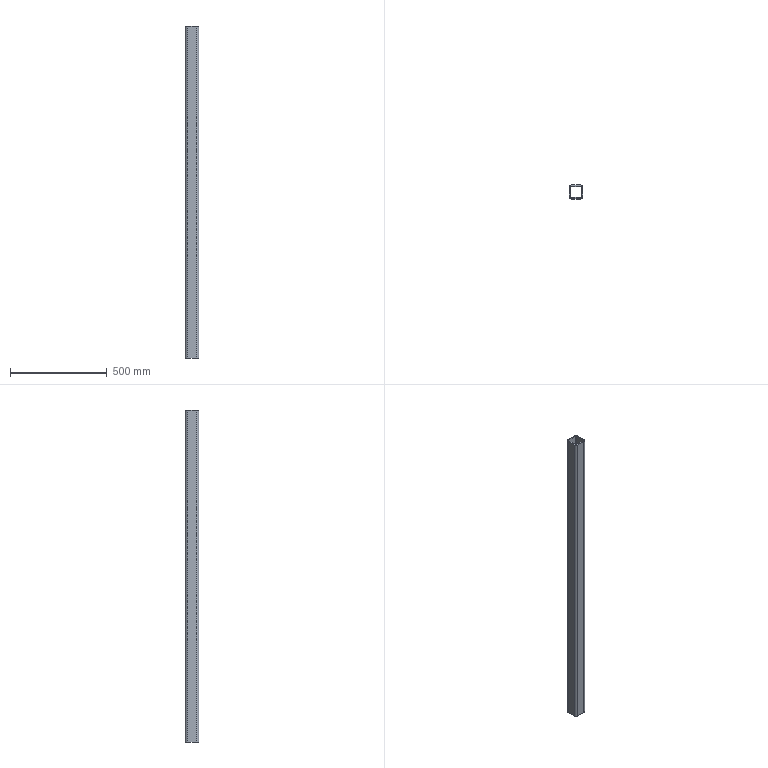Part | SolidWorks | features Extrusion 1 | 1 solid | 18 faces | box 70 x 70 x 1716 mm | volume 2476689 mm3 | plane 10 | cylinder 8 | commonest cylinder face diameters 12 x4 24 x4
STEP:
#1=CARTESIAN_POINT('',(0.,12.,1716.));
#2=VERTEX_POINT('',#1);
#3=CARTESIAN_POINT('',(12.,0.,1716.));
#4=VERTEX_POINT('',#3);
#5=CARTESIAN_POINT('',(12.,12.,1716.));
#6=DIRECTION('',(0.,0.,1.));
#7=DIRECTION('',(-1.,0.,0.));
#8=AXIS2_PLACEMENT_3D('',#5,#6,#7);
#9=CIRCLE('',#8,12.);
#10=EDGE_CURVE('',#2,#4,#9,.T.);
#11=ORIENTED_EDGE('',*,*,#10,.T.);
#12=CARTESIAN_POINT('',(58.,0.,1716.));
#13=VERTEX_POINT('',#12);
#14=CARTESIAN_POINT('',(12.,0.,1716.));
#15=DIRECTION('',(1.,0.,0.));
#16=VECTOR('',#15,1000.);
#17=LINE('',#14,#16);
#18=EDGE_CURVE('',#4,#13,#17,.T.);
#19=ORIENTED_EDGE('',*,*,#18,.T.);
#20=CARTESIAN_POINT('',(70.,12.,1716.));
#21=VERTEX_POINT('',#20);
#22=CARTESIAN_POINT('',(58.,12.,1716.));
#23=DIRECTION('',(0.,0.,1.));
#24=DIRECTION('',(1.,0.,0.));
#25=AXIS2_PLACEMENT_3D('',#22,#23,#24);
#26=CIRCLE('',#25,12.);
#27=EDGE_CURVE('',#13,#21,#26,.T.);
#28=ORIENTED_EDGE('',*,*,#27,.T.);
#29=CARTESIAN_POINT('',(70.,58.,1716.));
#30=VERTEX_POINT('',#29);
#31=CARTESIAN_POINT('',(70.,12.,1716.));
#32=DIRECTION('',(0.,1.,0.));
#33=VECTOR('',#32,1000.);
#34=LINE('',#31,#33);
#35=EDGE_CURVE('',#21,#30,#34,.T.);
#36=ORIENTED_EDGE('',*,*,#35,.T.);
#37=CARTESIAN_POINT('',(58.,70.,1716.));
#38=VERTEX_POINT('',#37);
#39=CARTESIAN_POINT('',(58.,58.,1716.));
#40=DIRECTION('',(0.,0.,1.));
#41=DIRECTION('',(-1.,0.,0.));
#42=AXIS2_PLACEMENT_3D('',#39,#40,#41);
#43=CIRCLE('',#42,12.);
#44=EDGE_CURVE('',#30,#38,#43,.T.);
#45=ORIENTED_EDGE('',*,*,#44,.T.);
#46=CARTESIAN_POINT('',(12.,70.,1716.));
#47=VERTEX_POINT('',#46);
#48=CARTESIAN_POINT('',(12.,70.,1716.));
#49=DIRECTION('',(-1.,0.,0.));
#50=VECTOR('',#49,1000.);
#51=LINE('',#48,#50);
#52=EDGE_CURVE('',#38,#47,#51,.T.);
#53=ORIENTED_EDGE('',*,*,#52,.T.);
#54=CARTESIAN_POINT('',(0.,58.,1716.));
#55=VERTEX_POINT('',#54);
#56=CARTESIAN_POINT('',(12.,58.,1716.));
#57=DIRECTION('',(0.,0.,1.));
#58=DIRECTION('',(-1.,0.,0.));
#59=AXIS2_PLACEMENT_3D('',#56,#57,#58);
#60=CIRCLE('',#59,12.);
#61=EDGE_CURVE('',#47,#55,#60,.T.);
#62=ORIENTED_EDGE('',*,*,#61,.T.);
#63=CARTESIAN_POINT('',(0.,12.,1716.));
#64=DIRECTION('',(0.,-1.,0.));
#65=VECTOR('',#64,1000.);
#66=LINE('',#63,#65);
#67=EDGE_CURVE('',#55,#2,#66,.T.);
#68=ORIENTED_EDGE('',*,*,#67,.T.);
#69=EDGE_LOOP('',(#11,#19,#28,#36,#45,#53,#62,#68));
#70=FACE_OUTER_BOUND('',#69,.T.);
#71=CARTESIAN_POINT('',(6.,12.,1716.));
#72=VERTEX_POINT('',#71);
#73=CARTESIAN_POINT('',(12.,6.,1716.));
#74=VERTEX_POINT('',#73);
#75=CARTESIAN_POINT('',(12.,12.,1716.));
#76=DIRECTION('',(0.,0.,1.));
#77=DIRECTION('',(-1.,0.,0.));
#78=AXIS2_PLACEMENT_3D('',#75,#76,#77);
#79=CIRCLE('',#78,6.);
#80=EDGE_CURVE('',#72,#74,#79,.T.);
#81=ORIENTED_EDGE('',*,*,#80,.F.);
#82=CARTESIAN_POINT('',(6.,58.,1716.));
#83=VERTEX_POINT('',#82);
#84=CARTESIAN_POINT('',(6.,12.,1716.));
#85=DIRECTION('',(0.,-1.,0.));
#86=VECTOR('',#85,1000.);
#87=LINE('',#84,#86);
#88=EDGE_CURVE('',#83,#72,#87,.T.);
#89=ORIENTED_EDGE('',*,*,#88,.F.);
#90=CARTESIAN_POINT('',(12.,64.,1716.));
#91=VERTEX_POINT('',#90);
#92=CARTESIAN_POINT('',(12.,58.,1716.));
#93=DIRECTION('',(0.,0.,1.));
#94=DIRECTION('',(-1.,0.,0.));
#95=AXIS2_PLACEMENT_3D('',#92,#93,#94);
#96=CIRCLE('',#95,6.);
#97=EDGE_CURVE('',#91,#83,#96,.T.);
#98=ORIENTED_EDGE('',*,*,#97,.F.);
#99=CARTESIAN_POINT('',(58.,64.,1716.));
#100=VERTEX_POINT('',#99);
#101=CARTESIAN_POINT('',(12.,64.,1716.));
#102=DIRECTION('',(-1.,0.,0.));
#103=VECTOR('',#102,1000.);
#104=LINE('',#101,#103);
#105=EDGE_CURVE('',#100,#91,#104,.T.);
#106=ORIENTED_EDGE('',*,*,#105,.F.);
#107=CARTESIAN_POINT('',(64.,58.,1716.));
#108=VERTEX_POINT('',#107);
#109=CARTESIAN_POINT('',(58.,58.,1716.));
#110=DIRECTION('',(0.,0.,1.));
#111=DIRECTION('',(-1.,0.,0.));
#112=AXIS2_PLACEMENT_3D('',#109,#110,#111);
#113=CIRCLE('',#112,6.);
#114=EDGE_CURVE('',#108,#100,#113,.T.);
#115=ORIENTED_EDGE('',*,*,#114,.F.);
#116=CARTESIAN_POINT('',(64.,12.,1716.));
#117=VERTEX_POINT('',#116);
#118=CARTESIAN_POINT('',(64.,12.,1716.));
#119=DIRECTION('',(0.,1.,0.));
#120=VECTOR('',#119,1000.);
#121=LINE('',#118,#120);
#122=EDGE_CURVE('',#117,#108,#121,.T.);
#123=ORIENTED_EDGE('',*,*,#122,.F.);
#124=CARTESIAN_POINT('',(58.,6.,1716.));
#125=VERTEX_POINT('',#124);
#126=CARTESIAN_POINT('',(58.,12.,1716.));
#127=DIRECTION('',(0.,0.,1.));
#128=DIRECTION('',(1.,0.,0.));
#129=AXIS2_PLACEMENT_3D('',#126,#127,#128);
#130=CIRCLE('',#129,6.);
#131=EDGE_CURVE('',#125,#117,#130,.T.);
#132=ORIENTED_EDGE('',*,*,#131,.F.);
#133=CARTESIAN_POINT('',(12.,6.,1716.));
#134=DIRECTION('',(1.,0.,0.));
#135=VECTOR('',#134,1000.);
#136=LINE('',#133,#135);
#137=EDGE_CURVE('',#74,#125,#136,.T.);
#138=ORIENTED_EDGE('',*,*,#137,.F.);
#139=EDGE_LOOP('',(#81,#89,#98,#106,#115,#123,#132,#138));
#140=FACE_BOUND('',#139,.T.);
#141=CARTESIAN_POINT('',(12.,12.,1716.));
#142=DIRECTION('',(0.,0.,-1.));
#143=DIRECTION('',(-1.,0.,0.));
#144=AXIS2_PLACEMENT_3D('',#141,#142,#143);
#145=PLANE('',#144);
#146=ADVANCED_FACE('',(#70,#140),#145,.F.);
#147=CARTESIAN_POINT('',(0.,12.,0.));
#148=VERTEX_POINT('',#147);
#149=CARTESIAN_POINT('',(12.,0.,0.));
#150=VERTEX_POINT('',#149);
#151=CARTESIAN_POINT('',(12.,12.,0.));
#152=DIRECTION('',(0.,0.,1.));
#153=DIRECTION('',(-1.,0.,0.));
#154=AXIS2_PLACEMENT_3D('',#151,#152,#153);
#155=CIRCLE('',#154,12.);
#156=EDGE_CURVE('',#148,#150,#155,.T.);
#157=ORIENTED_EDGE('',*,*,#156,.F.);
#158=CARTESIAN_POINT('',(0.,58.,0.));
#159=VERTEX_POINT('',#158);
#160=CARTESIAN_POINT('',(0.,12.,0.));
#161=DIRECTION('',(0.,-1.,0.));
#162=VECTOR('',#161,1000.);
#163=LINE('',#160,#162);
#164=EDGE_CURVE('',#159,#148,#163,.T.);
#165=ORIENTED_EDGE('',*,*,#164,.F.);
#166=CARTESIAN_POINT('',(12.,70.,0.));
#167=VERTEX_POINT('',#166);
#168=CARTESIAN_POINT('',(12.,58.,0.));
#169=DIRECTION('',(0.,0.,1.));
#170=DIRECTION('',(-1.,0.,0.));
#171=AXIS2_PLACEMENT_3D('',#168,#169,#170);
#172=CIRCLE('',#171,12.);
#173=EDGE_CURVE('',#167,#159,#172,.T.);
#174=ORIENTED_EDGE('',*,*,#173,.F.);
#175=CARTESIAN_POINT('',(58.,70.,0.));
#176=VERTEX_POINT('',#175);
#177=CARTESIAN_POINT('',(12.,70.,0.));
#178=DIRECTION('',(-1.,0.,0.));
#179=VECTOR('',#178,1000.);
#180=LINE('',#177,#179);
#181=EDGE_CURVE('',#176,#167,#180,.T.);
#182=ORIENTED_EDGE('',*,*,#181,.F.);
#183=CARTESIAN_POINT('',(70.,58.,0.));
#184=VERTEX_POINT('',#183);
#185=CARTESIAN_POINT('',(58.,58.,0.));
#186=DIRECTION('',(0.,0.,1.));
#187=DIRECTION('',(-1.,0.,0.));
#188=AXIS2_PLACEMENT_3D('',#185,#186,#187);
#189=CIRCLE('',#188,12.);
#190=EDGE_CURVE('',#184,#176,#189,.T.);
#191=ORIENTED_EDGE('',*,*,#190,.F.);
#192=CARTESIAN_POINT('',(70.,12.,0.));
#193=VERTEX_POINT('',#192);
#194=CARTESIAN_POINT('',(70.,12.,0.));
#195=DIRECTION('',(0.,1.,0.));
#196=VECTOR('',#195,1000.);
#197=LINE('',#194,#196);
#198=EDGE_CURVE('',#193,#184,#197,.T.);
#199=ORIENTED_EDGE('',*,*,#198,.F.);
#200=CARTESIAN_POINT('',(58.,0.,0.));
#201=VERTEX_POINT('',#200);
#202=CARTESIAN_POINT('',(58.,12.,0.));
#203=DIRECTION('',(0.,0.,1.));
#204=DIRECTION('',(1.,0.,0.));
#205=AXIS2_PLACEMENT_3D('',#202,#203,#204);
#206=CIRCLE('',#205,12.);
#207=EDGE_CURVE('',#201,#193,#206,.T.);
#208=ORIENTED_EDGE('',*,*,#207,.F.);
#209=CARTESIAN_POINT('',(12.,0.,0.));
#210=DIRECTION('',(1.,0.,0.));
#211=VECTOR('',#210,1000.);
#212=LINE('',#209,#211);
#213=EDGE_CURVE('',#150,#201,#212,.T.);
#214=ORIENTED_EDGE('',*,*,#213,.F.);
#215=EDGE_LOOP('',(#157,#165,#174,#182,#191,#199,#208,#214));
#216=FACE_OUTER_BOUND('',#215,.T.);
#217=CARTESIAN_POINT('',(6.,58.,0.));
#218=VERTEX_POINT('',#217);
#219=CARTESIAN_POINT('',(6.,12.,0.));
#220=VERTEX_POINT('',#219);
#221=CARTESIAN_POINT('',(6.,12.,0.));
#222=DIRECTION('',(0.,-1.,0.));
#223=VECTOR('',#222,1000.);
#224=LINE('',#221,#223);
#225=EDGE_CURVE('',#218,#220,#224,.T.);
#226=ORIENTED_EDGE('',*,*,#225,.T.);
#227=CARTESIAN_POINT('',(12.,6.,0.));
#228=VERTEX_POINT('',#227);
#229=CARTESIAN_POINT('',(12.,12.,0.));
#230=DIRECTION('',(0.,0.,1.));
#231=DIRECTION('',(-1.,0.,0.));
#232=AXIS2_PLACEMENT_3D('',#229,#230,#231);
#233=CIRCLE('',#232,6.);
#234=EDGE_CURVE('',#220,#228,#233,.T.);
#235=ORIENTED_EDGE('',*,*,#234,.T.);
#236=CARTESIAN_POINT('',(58.,6.,0.));
#237=VERTEX_POINT('',#236);
#238=CARTESIAN_POINT('',(12.,6.,0.));
#239=DIRECTION('',(1.,0.,0.));
#240=VECTOR('',#239,1000.);
#241=LINE('',#238,#240);
#242=EDGE_CURVE('',#228,#237,#241,.T.);
#243=ORIENTED_EDGE('',*,*,#242,.T.);
#244=CARTESIAN_POINT('',(64.,12.,0.));
#245=VERTEX_POINT('',#244);
#246=CARTESIAN_POINT('',(58.,12.,0.));
#247=DIRECTION('',(0.,0.,1.));
#248=DIRECTION('',(1.,0.,0.));
#249=AXIS2_PLACEMENT_3D('',#246,#247,#248);
#250=CIRCLE('',#249,6.);
#251=EDGE_CURVE('',#237,#245,#250,.T.);
#252=ORIENTED_EDGE('',*,*,#251,.T.);
#253=CARTESIAN_POINT('',(64.,58.,0.));
#254=VERTEX_POINT('',#253);
#255=CARTESIAN_POINT('',(64.,12.,0.));
#256=DIRECTION('',(0.,1.,0.));
#257=VECTOR('',#256,1000.);
#258=LINE('',#255,#257);
#259=EDGE_CURVE('',#245,#254,#258,.T.);
#260=ORIENTED_EDGE('',*,*,#259,.T.);
#261=CARTESIAN_POINT('',(58.,64.,0.));
#262=VERTEX_POINT('',#261);
#263=CARTESIAN_POINT('',(58.,58.,0.));
#264=DIRECTION('',(0.,0.,1.));
#265=DIRECTION('',(-1.,0.,0.));
#266=AXIS2_PLACEMENT_3D('',#263,#264,#265);
#267=CIRCLE('',#266,6.);
#268=EDGE_CURVE('',#254,#262,#267,.T.);
#269=ORIENTED_EDGE('',*,*,#268,.T.);
#270=CARTESIAN_POINT('',(12.,64.,0.));
#271=VERTEX_POINT('',#270);
#272=CARTESIAN_POINT('',(12.,64.,0.));
#273=DIRECTION('',(-1.,0.,0.));
#274=VECTOR('',#273,1000.);
#275=LINE('',#272,#274);
#276=EDGE_CURVE('',#262,#271,#275,.T.);
#277=ORIENTED_EDGE('',*,*,#276,.T.);
#278=CARTESIAN_POINT('',(12.,58.,0.));
#279=DIRECTION('',(0.,0.,1.));
#280=DIRECTION('',(-1.,0.,0.));
#281=AXIS2_PLACEMENT_3D('',#278,#279,#280);
#282=CIRCLE('',#281,6.);
#283=EDGE_CURVE('',#271,#218,#282,.T.);
#284=ORIENTED_EDGE('',*,*,#283,.T.);
#285=EDGE_LOOP('',(#226,#235,#243,#252,#260,#269,#277,#284));
#286=FACE_BOUND('',#285,.T.);
#287=CARTESIAN_POINT('',(12.,12.,0.));
#288=DIRECTION('',(0.,0.,-1.));
#289=DIRECTION('',(-1.,0.,0.));
#290=AXIS2_PLACEMENT_3D('',#287,#288,#289);
#291=PLANE('',#290);
#292=ADVANCED_FACE('',(#216,#286),#291,.T.);
#293=ORIENTED_EDGE('',*,*,#156,.T.);
#294=CARTESIAN_POINT('',(12.,0.,1716.));
#295=DIRECTION('',(0.,0.,-1.));
#296=VECTOR('',#295,1000.);
#297=LINE('',#294,#296);
#298=EDGE_CURVE('',#4,#150,#297,.T.);
#299=ORIENTED_EDGE('',*,*,#298,.F.);
#300=ORIENTED_EDGE('',*,*,#10,.F.);
#301=CARTESIAN_POINT('',(0.,12.,1716.));
#302=DIRECTION('',(0.,0.,-1.));
#303=VECTOR('',#302,1000.);
#304=LINE('',#301,#303);
#305=EDGE_CURVE('',#2,#148,#304,.T.);
#306=ORIENTED_EDGE('',*,*,#305,.T.);
#307=EDGE_LOOP('',(#293,#299,#300,#306));
#308=FACE_OUTER_BOUND('',#307,.T.);
#309=CARTESIAN_POINT('',(12.,12.,1716.));
#310=DIRECTION('',(0.,0.,-1.));
#311=DIRECTION('',(-1.,0.,0.));
#312=AXIS2_PLACEMENT_3D('',#309,#310,#311);
#313=CYLINDRICAL_SURFACE('',#312,12.);
#314=ADVANCED_FACE('',(#308),#313,.T.);
#315=ORIENTED_EDGE('',*,*,#213,.T.);
#316=CARTESIAN_POINT('',(58.,0.,1716.));
#317=DIRECTION('',(0.,0.,-1.));
#318=VECTOR('',#317,1000.);
#319=LINE('',#316,#318);
#320=EDGE_CURVE('',#13,#201,#319,.T.);
#321=ORIENTED_EDGE('',*,*,#320,.F.);
#322=ORIENTED_EDGE('',*,*,#18,.F.);
#323=ORIENTED_EDGE('',*,*,#298,.T.);
#324=EDGE_LOOP('',(#315,#321,#322,#323));
#325=FACE_OUTER_BOUND('',#324,.T.);
#326=CARTESIAN_POINT('',(12.,0.,1716.));
#327=DIRECTION('',(0.,1.,0.));
#328=DIRECTION('',(0.,0.,1.));
#329=AXIS2_PLACEMENT_3D('',#326,#327,#328);
#330=PLANE('',#329);
#331=ADVANCED_FACE('',(#325),#330,.F.);
#332=ORIENTED_EDGE('',*,*,#207,.T.);
#333=CARTESIAN_POINT('',(70.,12.,1716.));
#334=DIRECTION('',(0.,0.,-1.));
#335=VECTOR('',#334,1000.);
#336=LINE('',#333,#335);
#337=EDGE_CURVE('',#21,#193,#336,.T.);
#338=ORIENTED_EDGE('',*,*,#337,.F.);
#339=ORIENTED_EDGE('',*,*,#27,.F.);
#340=ORIENTED_EDGE('',*,*,#320,.T.);
#341=EDGE_LOOP('',(#332,#338,#339,#340));
#342=FACE_OUTER_BOUND('',#341,.T.);
#343=CARTESIAN_POINT('',(58.,12.,1716.));
#344=DIRECTION('',(0.,0.,-1.));
#345=DIRECTION('',(-1.,0.,0.));
#346=AXIS2_PLACEMENT_3D('',#343,#344,#345);
#347=CYLINDRICAL_SURFACE('',#346,12.);
#348=ADVANCED_FACE('',(#342),#347,.T.);
#349=ORIENTED_EDGE('',*,*,#198,.T.);
#350=CARTESIAN_POINT('',(70.,58.,1716.));
#351=DIRECTION('',(0.,0.,-1.));
#352=VECTOR('',#351,1000.);
#353=LINE('',#350,#352);
#354=EDGE_CURVE('',#30,#184,#353,.T.);
#355=ORIENTED_EDGE('',*,*,#354,.F.);
#356=ORIENTED_EDGE('',*,*,#35,.F.);
#357=ORIENTED_EDGE('',*,*,#337,.T.);
#358=EDGE_LOOP('',(#349,#355,#356,#357));
#359=FACE_OUTER_BOUND('',#358,.T.);
#360=CARTESIAN_POINT('',(70.,12.,1716.));
#361=DIRECTION('',(-1.,0.,0.));
#362=DIRECTION('',(0.,0.,1.));
#363=AXIS2_PLACEMENT_3D('',#360,#361,#362);
#364=PLANE('',#363);
#365=ADVANCED_FACE('',(#359),#364,.F.);
#366=ORIENTED_EDGE('',*,*,#190,.T.);
#367=CARTESIAN_POINT('',(58.,70.,1716.));
#368=DIRECTION('',(0.,0.,-1.));
#369=VECTOR('',#368,1000.);
#370=LINE('',#367,#369);
#371=EDGE_CURVE('',#38,#176,#370,.T.);
#372=ORIENTED_EDGE('',*,*,#371,.F.);
#373=ORIENTED_EDGE('',*,*,#44,.F.);
#374=ORIENTED_EDGE('',*,*,#354,.T.);
#375=EDGE_LOOP('',(#366,#372,#373,#374));
#376=FACE_OUTER_BOUND('',#375,.T.);
#377=CARTESIAN_POINT('',(58.,58.,1716.));
#378=DIRECTION('',(0.,0.,-1.));
#379=DIRECTION('',(-1.,0.,0.));
#380=AXIS2_PLACEMENT_3D('',#377,#378,#379);
#381=CYLINDRICAL_SURFACE('',#380,12.);
#382=ADVANCED_FACE('',(#376),#381,.T.);
#383=ORIENTED_EDGE('',*,*,#181,.T.);
#384=CARTESIAN_POINT('',(12.,70.,1716.));
#385=DIRECTION('',(0.,0.,-1.));
#386=VECTOR('',#385,1000.);
#387=LINE('',#384,#386);
#388=EDGE_CURVE('',#47,#167,#387,.T.);
#389=ORIENTED_EDGE('',*,*,#388,.F.);
#390=ORIENTED_EDGE('',*,*,#52,.F.);
#391=ORIENTED_EDGE('',*,*,#371,.T.);
#392=EDGE_LOOP('',(#383,#389,#390,#391));
#393=FACE_OUTER_BOUND('',#392,.T.);
#394=CARTESIAN_POINT('',(12.,70.,1716.));
#395=DIRECTION('',(0.,-1.,0.));
#396=DIRECTION('',(0.,0.,-1.));
#397=AXIS2_PLACEMENT_3D('',#394,#395,#396);
#398=PLANE('',#397);
#399=ADVANCED_FACE('',(#393),#398,.F.);
#400=ORIENTED_EDGE('',*,*,#173,.T.);
#401=CARTESIAN_POINT('',(0.,58.,1716.));
#402=DIRECTION('',(0.,0.,-1.));
#403=VECTOR('',#402,1000.);
#404=LINE('',#401,#403);
#405=EDGE_CURVE('',#55,#159,#404,.T.);
#406=ORIENTED_EDGE('',*,*,#405,.F.);
#407=ORIENTED_EDGE('',*,*,#61,.F.);
#408=ORIENTED_EDGE('',*,*,#388,.T.);
#409=EDGE_LOOP('',(#400,#406,#407,#408));
#410=FACE_OUTER_BOUND('',#409,.T.);
#411=CARTESIAN_POINT('',(12.,58.,1716.));
#412=DIRECTION('',(0.,0.,-1.));
#413=DIRECTION('',(-1.,0.,0.));
#414=AXIS2_PLACEMENT_3D('',#411,#412,#413);
#415=CYLINDRICAL_SURFACE('',#414,12.);
#416=ADVANCED_FACE('',(#410),#415,.T.);
#417=ORIENTED_EDGE('',*,*,#164,.T.);
#418=ORIENTED_EDGE('',*,*,#305,.F.);
#419=ORIENTED_EDGE('',*,*,#67,.F.);
#420=ORIENTED_EDGE('',*,*,#405,.T.);
#421=EDGE_LOOP('',(#417,#418,#419,#420));
#422=FACE_OUTER_BOUND('',#421,.T.);
#423=CARTESIAN_POINT('',(0.,12.,1716.));
#424=DIRECTION('',(1.,0.,0.));
#425=DIRECTION('',(0.,0.,-1.));
#426=AXIS2_PLACEMENT_3D('',#423,#424,#425);
#427=PLANE('',#426);
#428=ADVANCED_FACE('',(#422),#427,.F.);
#429=ORIENTED_EDGE('',*,*,#234,.F.);
#430=CARTESIAN_POINT('',(6.,12.,1716.));
#431=DIRECTION('',(0.,0.,-1.));
#432=VECTOR('',#431,1000.);
#433=LINE('',#430,#432);
#434=EDGE_CURVE('',#72,#220,#433,.T.);
#435=ORIENTED_EDGE('',*,*,#434,.F.);
#436=ORIENTED_EDGE('',*,*,#80,.T.);
#437=CARTESIAN_POINT('',(12.,6.,1716.));
#438=DIRECTION('',(0.,0.,-1.));
#439=VECTOR('',#438,1000.);
#440=LINE('',#437,#439);
#441=EDGE_CURVE('',#74,#228,#440,.T.);
#442=ORIENTED_EDGE('',*,*,#441,.T.);
#443=EDGE_LOOP('',(#429,#435,#436,#442));
#444=FACE_OUTER_BOUND('',#443,.T.);
#445=CARTESIAN_POINT('',(12.,12.,1716.));
#446=DIRECTION('',(0.,0.,-1.));
#447=DIRECTION('',(-1.,0.,0.));
#448=AXIS2_PLACEMENT_3D('',#445,#446,#447);
#449=CYLINDRICAL_SURFACE('',#448,6.);
#450=ADVANCED_FACE('',(#444),#449,.F.);
#451=ORIENTED_EDGE('',*,*,#242,.F.);
#452=ORIENTED_EDGE('',*,*,#441,.F.);
#453=ORIENTED_EDGE('',*,*,#137,.T.);
#454=CARTESIAN_POINT('',(58.,6.,1716.));
#455=DIRECTION('',(0.,0.,-1.));
#456=VECTOR('',#455,1000.);
#457=LINE('',#454,#456);
#458=EDGE_CURVE('',#125,#237,#457,.T.);
#459=ORIENTED_EDGE('',*,*,#458,.T.);
#460=EDGE_LOOP('',(#451,#452,#453,#459));
#461=FACE_OUTER_BOUND('',#460,.T.);
#462=CARTESIAN_POINT('',(12.,6.,1716.));
#463=DIRECTION('',(0.,1.,0.));
#464=DIRECTION('',(0.,0.,1.));
#465=AXIS2_PLACEMENT_3D('',#462,#463,#464);
#466=PLANE('',#465);
#467=ADVANCED_FACE('',(#461),#466,.T.);
#468=ORIENTED_EDGE('',*,*,#251,.F.);
#469=ORIENTED_EDGE('',*,*,#458,.F.);
#470=ORIENTED_EDGE('',*,*,#131,.T.);
#471=CARTESIAN_POINT('',(64.,12.,1716.));
#472=DIRECTION('',(0.,0.,-1.));
#473=VECTOR('',#472,1000.);
#474=LINE('',#471,#473);
#475=EDGE_CURVE('',#117,#245,#474,.T.);
#476=ORIENTED_EDGE('',*,*,#475,.T.);
#477=EDGE_LOOP('',(#468,#469,#470,#476));
#478=FACE_OUTER_BOUND('',#477,.T.);
#479=CARTESIAN_POINT('',(58.,12.,1716.));
#480=DIRECTION('',(0.,0.,-1.));
#481=DIRECTION('',(-1.,0.,0.));
#482=AXIS2_PLACEMENT_3D('',#479,#480,#481);
#483=CYLINDRICAL_SURFACE('',#482,6.);
#484=ADVANCED_FACE('',(#478),#483,.F.);
#485=ORIENTED_EDGE('',*,*,#259,.F.);
#486=ORIENTED_EDGE('',*,*,#475,.F.);
#487=ORIENTED_EDGE('',*,*,#122,.T.);
#488=CARTESIAN_POINT('',(64.,58.,1716.));
#489=DIRECTION('',(0.,0.,-1.));
#490=VECTOR('',#489,1000.);
#491=LINE('',#488,#490);
#492=EDGE_CURVE('',#108,#254,#491,.T.);
#493=ORIENTED_EDGE('',*,*,#492,.T.);
#494=EDGE_LOOP('',(#485,#486,#487,#493));
#495=FACE_OUTER_BOUND('',#494,.T.);
#496=CARTESIAN_POINT('',(64.,12.,1716.));
#497=DIRECTION('',(-1.,0.,0.));
#498=DIRECTION('',(0.,0.,1.));
#499=AXIS2_PLACEMENT_3D('',#496,#497,#498);
#500=PLANE('',#499);
#501=ADVANCED_FACE('',(#495),#500,.T.);
#502=ORIENTED_EDGE('',*,*,#268,.F.);
#503=ORIENTED_EDGE('',*,*,#492,.F.);
#504=ORIENTED_EDGE('',*,*,#114,.T.);
#505=CARTESIAN_POINT('',(58.,64.,1716.));
#506=DIRECTION('',(0.,0.,-1.));
#507=VECTOR('',#506,1000.);
#508=LINE('',#505,#507);
#509=EDGE_CURVE('',#100,#262,#508,.T.);
#510=ORIENTED_EDGE('',*,*,#509,.T.);
#511=EDGE_LOOP('',(#502,#503,#504,#510));
#512=FACE_OUTER_BOUND('',#511,.T.);
#513=CARTESIAN_POINT('',(58.,58.,1716.));
#514=DIRECTION('',(0.,0.,-1.));
#515=DIRECTION('',(-1.,0.,0.));
#516=AXIS2_PLACEMENT_3D('',#513,#514,#515);
#517=CYLINDRICAL_SURFACE('',#516,6.);
#518=ADVANCED_FACE('',(#512),#517,.F.);
#519=ORIENTED_EDGE('',*,*,#276,.F.);
#520=ORIENTED_EDGE('',*,*,#509,.F.);
#521=ORIENTED_EDGE('',*,*,#105,.T.);
#522=CARTESIAN_POINT('',(12.,64.,1716.));
#523=DIRECTION('',(0.,0.,-1.));
#524=VECTOR('',#523,1000.);
#525=LINE('',#522,#524);
#526=EDGE_CURVE('',#91,#271,#525,.T.);
#527=ORIENTED_EDGE('',*,*,#526,.T.);
#528=EDGE_LOOP('',(#519,#520,#521,#527));
#529=FACE_OUTER_BOUND('',#528,.T.);
#530=CARTESIAN_POINT('',(12.,64.,1716.));
#531=DIRECTION('',(0.,-1.,0.));
#532=DIRECTION('',(0.,0.,-1.));
#533=AXIS2_PLACEMENT_3D('',#530,#531,#532);
#534=PLANE('',#533);
#535=ADVANCED_FACE('',(#529),#534,.T.);
#536=ORIENTED_EDGE('',*,*,#283,.F.);
#537=ORIENTED_EDGE('',*,*,#526,.F.);
#538=ORIENTED_EDGE('',*,*,#97,.T.);
#539=CARTESIAN_POINT('',(6.,58.,1716.));
#540=DIRECTION('',(0.,0.,-1.));
#541=VECTOR('',#540,1000.);
#542=LINE('',#539,#541);
#543=EDGE_CURVE('',#83,#218,#542,.T.);
#544=ORIENTED_EDGE('',*,*,#543,.T.);
#545=EDGE_LOOP('',(#536,#537,#538,#544));
#546=FACE_OUTER_BOUND('',#545,.T.);
#547=CARTESIAN_POINT('',(12.,58.,1716.));
#548=DIRECTION('',(0.,0.,-1.));
#549=DIRECTION('',(-1.,0.,0.));
#550=AXIS2_PLACEMENT_3D('',#547,#548,#549);
#551=CYLINDRICAL_SURFACE('',#550,6.);
#552=ADVANCED_FACE('',(#546),#551,.F.);
#553=ORIENTED_EDGE('',*,*,#225,.F.);
#554=ORIENTED_EDGE('',*,*,#543,.F.);
#555=ORIENTED_EDGE('',*,*,#88,.T.);
#556=ORIENTED_EDGE('',*,*,#434,.T.);
#557=EDGE_LOOP('',(#553,#554,#555,#556));
#558=FACE_OUTER_BOUND('',#557,.T.);
#559=CARTESIAN_POINT('',(6.,12.,1716.));
#560=DIRECTION('',(1.,0.,0.));
#561=DIRECTION('',(0.,0.,-1.));
#562=AXIS2_PLACEMENT_3D('',#559,#560,#561);
#563=PLANE('',#562);
#564=ADVANCED_FACE('',(#558),#563,.T.);
#565=CLOSED_SHELL('',(#146,#292,#314,#331,#348,#365,#382,#399,#416,#428,#450,#467,#484,#501,#518,#535,#552,#564));
#566=MANIFOLD_SOLID_BREP('',#565);
#567=CARTESIAN_POINT('',(0.,0.,0.));
#568=DIRECTION('',(0.,0.,1.));
#569=DIRECTION('',(1.,0.,0.));
#570=AXIS2_PLACEMENT_3D('',#567,#568,#569);
#571=(LENGTH_UNIT()NAMED_UNIT(*)SI_UNIT(.MILLI.,.METRE.));
#572=UNCERTAINTY_MEASURE_WITH_UNIT(LENGTH_MEASURE(0.00001),#571,'','');
#573=(NAMED_UNIT(*)PLANE_ANGLE_UNIT()SI_UNIT($,.RADIAN.));
#574=(NAMED_UNIT(*)SI_UNIT($,.STERADIAN.)SOLID_ANGLE_UNIT());
#575=(GEOMETRIC_REPRESENTATION_CONTEXT(3)GLOBAL_UNCERTAINTY_ASSIGNED_CONTEXT((#572))GLOBAL_UNIT_ASSIGNED_CONTEXT((#571,#573,#574))REPRESENTATION_CONTEXT('',''));
#576=ADVANCED_BREP_SHAPE_REPRESENTATION('',(#566,#570),#575);